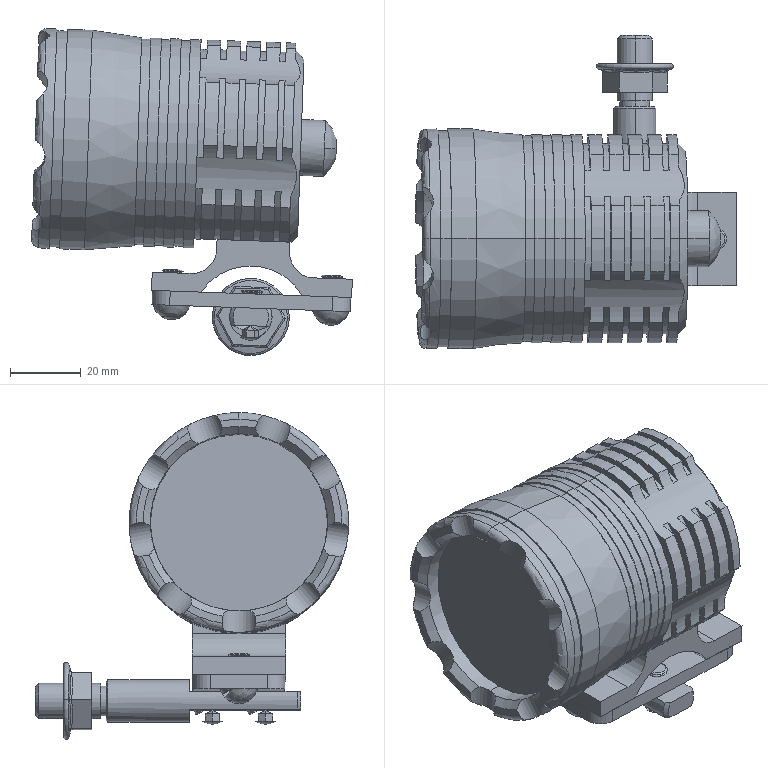Part | SolidWorks | features BaseBody 1 | 1 solid | 525 faces | box 90.524 x 88.5 x 92.29 mm | volume 183174 mm3 | plane 178 | cylinder 165 | cone 126 | sphere 26 | spline 18 | torus 12 | commonest cylinder face diameters 6 x48 58.8 x36 53.718 x25 10.407 x9 6.5 x8 10 x8